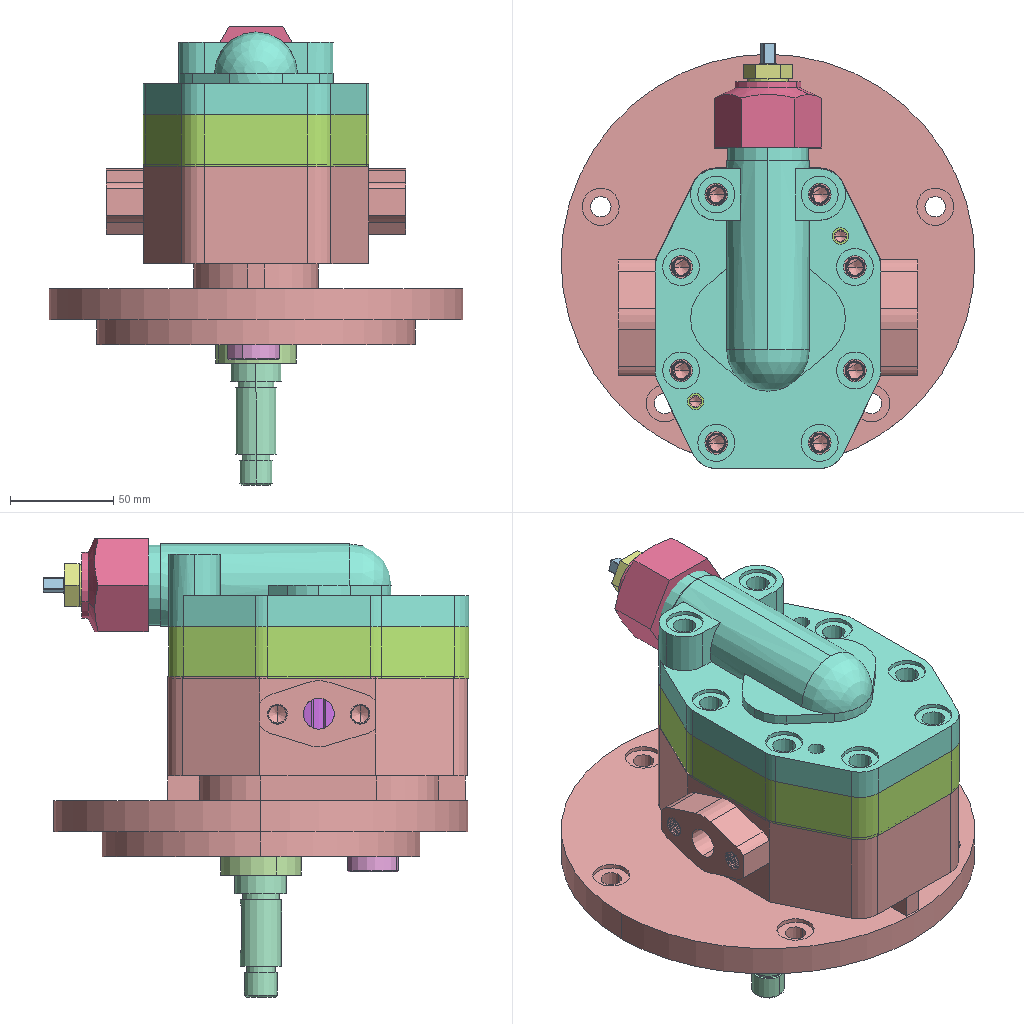Assembly | SolidWorks | 16 different items | 17 placed | box 200 x 206 x 222 mm
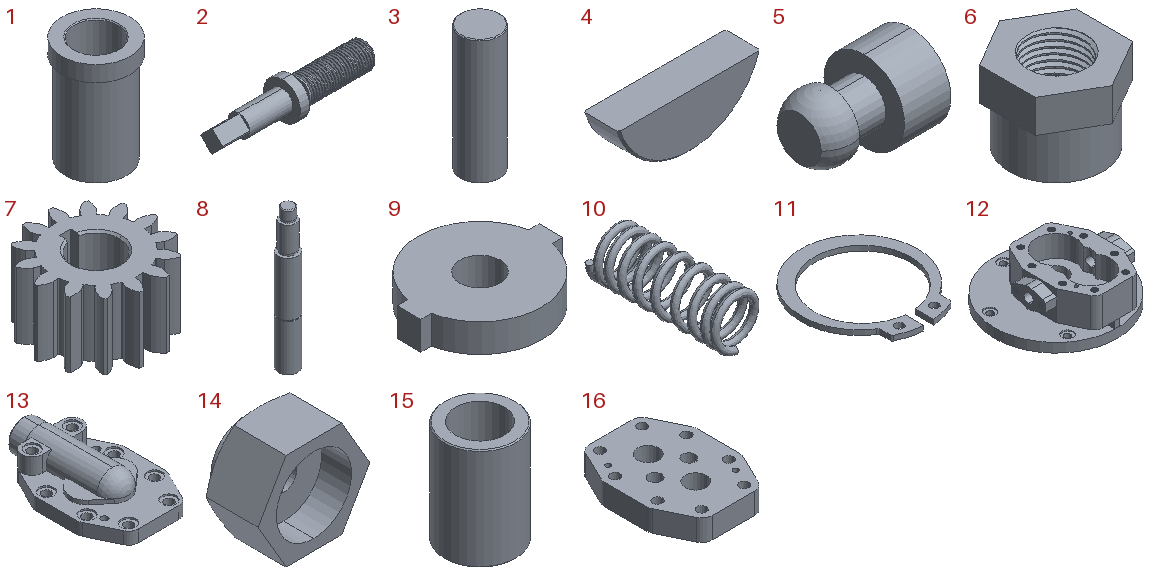Parts list (item | quantity | size | volume | features):
1 | x1 | 39 x 39 x 60 mm | 30347 mm3 | features Revolution 1
2 | x1 | 56.6 x 13.6 x 13.6 mm | 3300 mm3 | features ICE 5, Chamfer 1, Revolution 1, SweepThread 1
3 | x1 | 25 x 25 x 80 mm | 39251 mm3 | features Revolution 1
4 | x1 | 24 x 6 x 9 mm | 951.697 mm3 | features Chamfer 1, Extrusion 1
5 | x1 | 36 x 26 x 26 mm | 7859 mm3 | features Revolution 1
6 | x1 | 20.8 x 24.018 x 17 mm | 3648 mm3 | features HoleWzd 1, ICE 1, Revolution 1, SweepThread 1
7 | x2 | 64 x 62.751 x 35 mm | 62928 mm3 | features BaseBody 1, Chamfer 1, Fillet 1, ICE 1, RevCut 1
8 | x1 | 25 x 25 x 180 mm | 76361 mm3 | features Chamfer 1, ICE 1, RefSurface 1, Revolution 1, ThickenCut 1
9 | x1 | 30 x 26 x 6 mm | 2970 mm3 | features Extrusion 1
10 | x1 | 22 x 58 x 22 mm | 3891 mm3 | features Helix 1, Sweep 1
11 | x1 | 28.2 x 30.881 x 1.2 mm | 270.476 mm3 | features Extrusion 1
12 | x1 | 200 x 200 x 87 mm | 962197 mm3 | features SweepThread 12, ICE 11, HoleWzd 3, MirrorPattern 2, Rib 2, 3DProfileFeature 1, Extrusion 1
13 | x1 | 109 x 169 x 40 mm | 262615 mm3 | features ICE 13, 3DProfileFeature 1, Dome 1, HoleWzd 1, MirrorPattern 1, StudWizard 1
14 | x1 | 51.962 x 32 x 45 mm | 33727 mm3 | features ICE 7
15 | x1 | 35 x 35 x 50 mm | 24381 mm3 | features Revolution 1
16 | x1 | 109 x 145 x 25 mm | 291332 mm3 | features ICE 3, Extrusion 1, MirrorPattern 1
Mates (type | each side: item.copy, entity, surface, feature):
Concentric | 12.1 face cylinder Cut-Extrude4 | 15.1 face cylinder Revolve1
Coincident | 12.1 face plane Cut-Extrude3 | 15.1 face plane Revolve1
Concentric | 15.1 face cylinder Revolve1 | assembly face
Coincident | 12.1 face plane Cut-Extrude3 | assembly face
Parallel | 12.1 face plane Boss-Extrude4 | 13.1 face plane Boss-Extrude7
Concentric | 13.1 face cylinder Cut-Extrude5 | 5.1 face cylinder Revolve1
Coincident | 13.1 face plane Cut-Extrude6 | 5.1 face plane Revolve1
Concentric | 13.1 face cylinder Cut-Extrude5 | 9.1 face cylinder Boss-Extrude1
Parallel | 13.1 face plane Cut-Extrude8 | 9.1 face plane Boss-Extrude1
Concentric | 13.1 edge | 14.1 face cylinder Cut-Extrude1
Coincident | 13.1 face plane Boss-Extrude6 | 14.1 face plane Cut-Extrude1
Concentric | 14.1 face cylinder Cut-Extrude2 | 2.1 face cylinder Boss-Extrude1
Concentric | 14.1 face cylinder Cut-Extrude2 | 6.1 face cylinder Revolve1
Parallel | 14.1 face plane Boss-Extrude1 | 6.1 face plane Boss-Extrude1
Concentric | 12.1 face cylinder Cut-Extrude4 | 7.1 face cylinder Cut-Revolve1
GearDim | 7.1 face cylinder Cut-Revolve1 | 7.2 face cylinder Cut-Revolve1
Coincident | 7.1 face plane Input4 | 7.2 face plane Input4
Concentric | 8.1 face cylinder Cut-Thicken1 | 4.1 face cylinder Boss-Extrude1
Parallel | 8.1 face plane Cut-Extrude1 | 4.1 face plane Boss-Extrude1
Coincident | 8.1 face plane Cut-Thicken1 | 4.1 face plane Boss-Extrude1
Concentric | 12.1 face cylinder Cut-Extrude4 | 8.1 face cylinder Revolve1
Parallel | 12.1 face plane Boss-Extrude9 | 8.1 face plane Cut-Extrude1
Concentric | 7.2 edge | 8.1 face cylinder Revolve1
Coincident | 7.2 face plane Cut-Extrude1 | 4.1 face plane Boss-Extrude1
Coincident | 12.1 face plane Cut-Extrude3 | 7.2 face plane Input4
Concentric | 8.1 face cylinder Revolve1 | 11.1 edge
Coincident | 8.1 face plane Revolve1 | 11.1 face plane Boss-Extrude1
Coincident | 7.2 face plane Input4 | 11.1 face plane Boss-Extrude1
Parallel | 12.1 face plane Boss-Extrude4 | 7.2 face plane Cut-Extrude1
Coincident | 12.1 face plane Boss-Extrude2 | 1.1 face plane Revolve1
Concentric | 8.1 face cylinder Revolve1 | 1.1 face cylinder Revolve1
Concentric | 13.1 face cylinder Cut-Extrude4 | assembly face | 2 times
Coincident | 12.1 face cone Tap Drill for M10 Tap3 | assembly edge
Concentric | 12.1 face cone Tap Drill for M10 Tap3 | assembly face
Concentric | 13.1 face cylinder Mirror1 | assembly face | 5 times
Concentric | 13.1 select_type:24 | assembly face | 2 times
Parallel | assembly face | assembly face | 6 times
Concentric | 12.1 face cylinder Tap Drill for M6 Tap1 | 16.1 face cylinder Cut-Extrude5
Concentric | 12.1 face cylinder Tap Drill for M6 Tap1 | 16.1 face cylinder Cut-Extrude7
Coincident | 16.1 face plane Boss-Extrude2 | 13.1 face plane Boss-Extrude3
Concentric | 12.1 edge | assembly face
Concentric | 12.1 face cylinder Tap Drill for M6 Tap1 | assembly edge
Concentric | 13.1 face cylinder Cut-Extrude11 | assembly face | 2 times
Coincident | assembly face | assembly face | 2 times
Coincident | 13.1 face plane Boss-Extrude4 | assembly face
Coincident | 12.1 face plane Boss-Extrude2 | assembly face
Concentric | 15.1 edge | assembly face
Concentric | 13.1 edge | assembly edge | 2 times
Coincident | 13.1 face plane Mirror1 | assembly face
Coincident | 13.1 face plane Cut-Extrude3 | assembly face
Concentric | assembly edge | assembly edge | 2 times